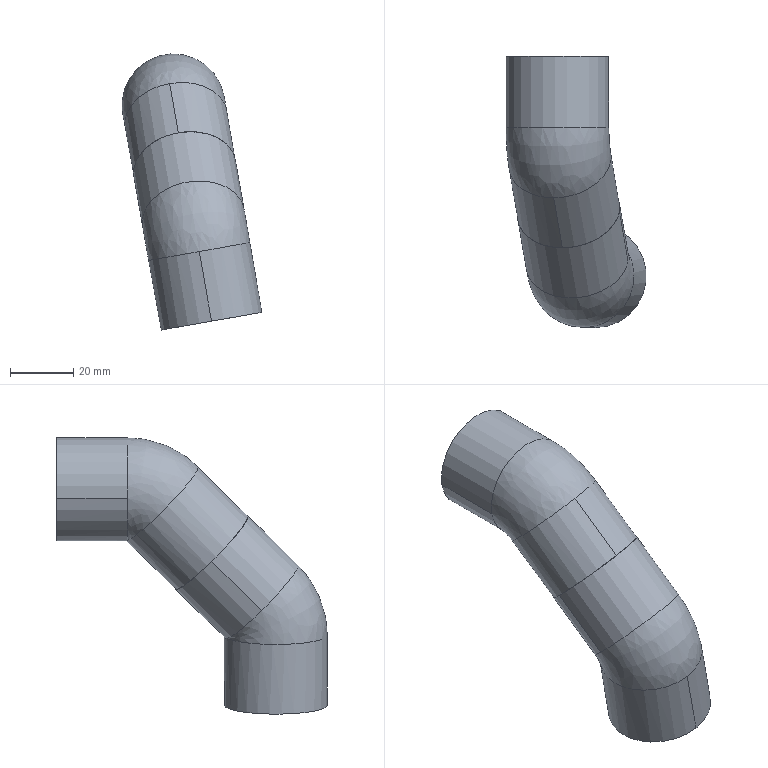Part | SolidWorks | 2 solids | 30 faces | box 44.298 x 85.549 x 87.319 mm | volume 55176 mm3 | plane 8 | cone 8 | cylinder 8 | torus 4 | spline 2 | commonest cylinder face diameters 32.512 x8